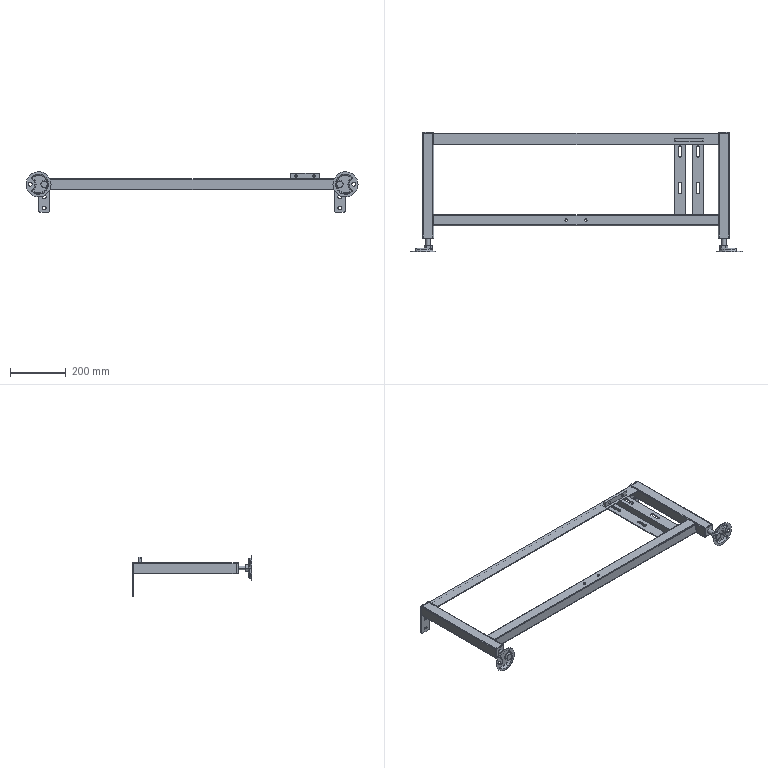Part | SolidWorks | 13 solids | 357 faces | box 1190 x 430 x 145 mm | volume 955043 mm3 | plane 160 | cylinder 121 | cone 40 | sphere 16 | torus 12 | spline 8 | commonest cylinder face diameters 9 x22 6 x20 2 x14 10 x13 3 x12 11 x8